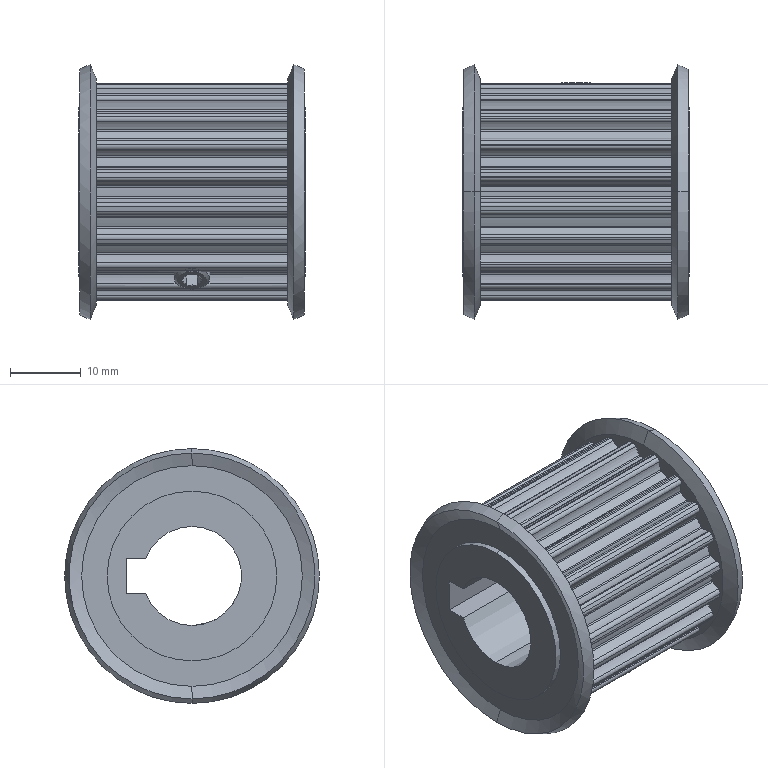Part | SolidWorks | features BaseBody 3 | 3 solids | 268 faces | box 32 x 36 x 36 mm | volume 16309 mm3 | cylinder 207 | cone 34 | plane 27 | commonest cylinder face diameters 0.5 x51 1.1 x50 6.55 x48 27.33 x23 30.87 x20 4.134 x4